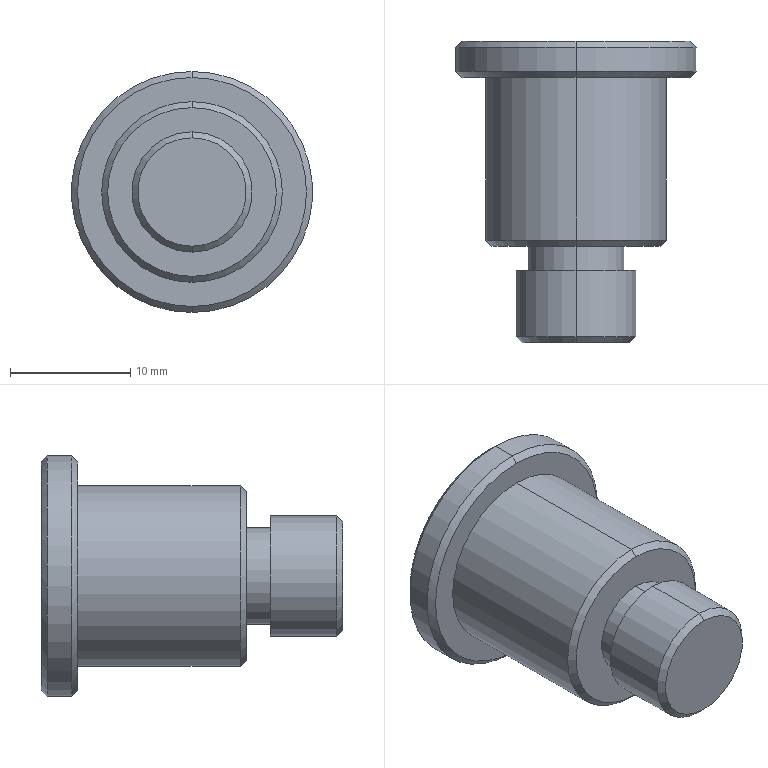Part | SolidWorks | features Chamfer 1, Revolution 1 | 1 solid | 21 faces | box 20 x 25 x 20 mm | volume 3963 mm3 | cone 8 | cylinder 8 | plane 5 | commonest cylinder face diameters 8 x2 10 x2 15 x2 20 x2
STEP:
#1=CARTESIAN_POINT('',(0.,-25.,-4.5));
#2=VERTEX_POINT('',#1);
#3=CARTESIAN_POINT('',(0.,-25.,4.5));
#4=VERTEX_POINT('',#3);
#5=CARTESIAN_POINT('',(0.,-25.,0.));
#6=DIRECTION('',(0.,-1.,0.));
#7=DIRECTION('',(0.,0.,1.));
#8=AXIS2_PLACEMENT_3D('',#5,#6,#7);
#9=CIRCLE('',#8,4.5);
#10=EDGE_CURVE('',#2,#4,#9,.T.);
#11=ORIENTED_EDGE('',*,*,#10,.F.);
#12=CARTESIAN_POINT('',(0.,-24.5,-5.));
#13=VERTEX_POINT('',#12);
#14=CARTESIAN_POINT('',(0.,-24.5,-5.));
#15=DIRECTION('',(0.,0.7071,-0.7071));
#16=VECTOR('',#15,1000.);
#17=LINE('',#14,#16);
#18=EDGE_CURVE('',#2,#13,#17,.T.);
#19=ORIENTED_EDGE('',*,*,#18,.T.);
#20=CARTESIAN_POINT('',(0.,-24.5,5.));
#21=VERTEX_POINT('',#20);
#22=CARTESIAN_POINT('',(0.,-24.5,0.));
#23=DIRECTION('',(0.,1.,0.));
#24=DIRECTION('',(0.,0.,1.));
#25=AXIS2_PLACEMENT_3D('',#22,#23,#24);
#26=CIRCLE('',#25,5.);
#27=EDGE_CURVE('',#21,#13,#26,.T.);
#28=ORIENTED_EDGE('',*,*,#27,.F.);
#29=CARTESIAN_POINT('',(0.,-24.5,5.));
#30=DIRECTION('',(0.,0.7071,0.7071));
#31=VECTOR('',#30,1000.);
#32=LINE('',#29,#31);
#33=EDGE_CURVE('',#4,#21,#32,.T.);
#34=ORIENTED_EDGE('',*,*,#33,.F.);
#35=EDGE_LOOP('',(#11,#19,#28,#34));
#36=FACE_OUTER_BOUND('',#35,.T.);
#37=CARTESIAN_POINT('',(0.,-24.5,0.));
#38=DIRECTION('',(0.,1.,0.));
#39=DIRECTION('',(0.,0.,1.));
#40=AXIS2_PLACEMENT_3D('',#37,#38,#39);
#41=CONICAL_SURFACE('',#40,5.,0.7854);
#42=ADVANCED_FACE('',(#36),#41,.T.);
#43=CARTESIAN_POINT('',(0.,-17.,-7.));
#44=VERTEX_POINT('',#43);
#45=CARTESIAN_POINT('',(0.,-17.,7.));
#46=VERTEX_POINT('',#45);
#47=CARTESIAN_POINT('',(0.,-17.,0.));
#48=DIRECTION('',(0.,-1.,0.));
#49=DIRECTION('',(0.,0.,1.));
#50=AXIS2_PLACEMENT_3D('',#47,#48,#49);
#51=CIRCLE('',#50,7.);
#52=EDGE_CURVE('',#44,#46,#51,.T.);
#53=ORIENTED_EDGE('',*,*,#52,.F.);
#54=CARTESIAN_POINT('',(0.,-16.5,-7.5));
#55=VERTEX_POINT('',#54);
#56=CARTESIAN_POINT('',(0.,-16.5,-7.5));
#57=DIRECTION('',(0.,0.7071,-0.7071));
#58=VECTOR('',#57,1000.);
#59=LINE('',#56,#58);
#60=EDGE_CURVE('',#44,#55,#59,.T.);
#61=ORIENTED_EDGE('',*,*,#60,.T.);
#62=CARTESIAN_POINT('',(0.,-16.5,7.5));
#63=VERTEX_POINT('',#62);
#64=CARTESIAN_POINT('',(0.,-16.5,0.));
#65=DIRECTION('',(0.,1.,0.));
#66=DIRECTION('',(0.,0.,1.));
#67=AXIS2_PLACEMENT_3D('',#64,#65,#66);
#68=CIRCLE('',#67,7.5);
#69=EDGE_CURVE('',#63,#55,#68,.T.);
#70=ORIENTED_EDGE('',*,*,#69,.F.);
#71=CARTESIAN_POINT('',(0.,-16.5,7.5));
#72=DIRECTION('',(0.,0.7071,0.7071));
#73=VECTOR('',#72,1000.);
#74=LINE('',#71,#73);
#75=EDGE_CURVE('',#46,#63,#74,.T.);
#76=ORIENTED_EDGE('',*,*,#75,.F.);
#77=EDGE_LOOP('',(#53,#61,#70,#76));
#78=FACE_OUTER_BOUND('',#77,.T.);
#79=CARTESIAN_POINT('',(0.,-16.5,0.));
#80=DIRECTION('',(0.,1.,0.));
#81=DIRECTION('',(0.,0.,1.));
#82=AXIS2_PLACEMENT_3D('',#79,#80,#81);
#83=CONICAL_SURFACE('',#82,7.5,0.7854);
#84=ADVANCED_FACE('',(#78),#83,.T.);
#85=CARTESIAN_POINT('',(0.,-3.,-9.5));
#86=VERTEX_POINT('',#85);
#87=CARTESIAN_POINT('',(0.,-3.,9.5));
#88=VERTEX_POINT('',#87);
#89=CARTESIAN_POINT('',(0.,-3.,0.));
#90=DIRECTION('',(0.,-1.,0.));
#91=DIRECTION('',(0.,0.,1.));
#92=AXIS2_PLACEMENT_3D('',#89,#90,#91);
#93=CIRCLE('',#92,9.5);
#94=EDGE_CURVE('',#86,#88,#93,.T.);
#95=ORIENTED_EDGE('',*,*,#94,.F.);
#96=CARTESIAN_POINT('',(0.,-2.5,-10.));
#97=VERTEX_POINT('',#96);
#98=CARTESIAN_POINT('',(0.,-2.5,-10.));
#99=DIRECTION('',(0.,0.7071,-0.7071));
#100=VECTOR('',#99,1000.);
#101=LINE('',#98,#100);
#102=EDGE_CURVE('',#86,#97,#101,.T.);
#103=ORIENTED_EDGE('',*,*,#102,.T.);
#104=CARTESIAN_POINT('',(0.,-2.5,10.));
#105=VERTEX_POINT('',#104);
#106=CARTESIAN_POINT('',(0.,-2.5,0.));
#107=DIRECTION('',(0.,1.,0.));
#108=DIRECTION('',(0.,0.,1.));
#109=AXIS2_PLACEMENT_3D('',#106,#107,#108);
#110=CIRCLE('',#109,10.);
#111=EDGE_CURVE('',#105,#97,#110,.T.);
#112=ORIENTED_EDGE('',*,*,#111,.F.);
#113=CARTESIAN_POINT('',(0.,-2.5,10.));
#114=DIRECTION('',(0.,0.7071,0.7071));
#115=VECTOR('',#114,1000.);
#116=LINE('',#113,#115);
#117=EDGE_CURVE('',#88,#105,#116,.T.);
#118=ORIENTED_EDGE('',*,*,#117,.F.);
#119=EDGE_LOOP('',(#95,#103,#112,#118));
#120=FACE_OUTER_BOUND('',#119,.T.);
#121=CARTESIAN_POINT('',(0.,-2.5,0.));
#122=DIRECTION('',(0.,1.,0.));
#123=DIRECTION('',(0.,0.,1.));
#124=AXIS2_PLACEMENT_3D('',#121,#122,#123);
#125=CONICAL_SURFACE('',#124,10.,0.7854);
#126=ADVANCED_FACE('',(#120),#125,.T.);
#127=CARTESIAN_POINT('',(0.,0.,9.5));
#128=VERTEX_POINT('',#127);
#129=CARTESIAN_POINT('',(0.,0.,-9.5));
#130=VERTEX_POINT('',#129);
#131=CARTESIAN_POINT('',(0.,0.,0.));
#132=DIRECTION('',(0.,1.,0.));
#133=DIRECTION('',(0.,0.,-1.));
#134=AXIS2_PLACEMENT_3D('',#131,#132,#133);
#135=CIRCLE('',#134,9.5);
#136=EDGE_CURVE('',#128,#130,#135,.T.);
#137=ORIENTED_EDGE('',*,*,#136,.F.);
#138=CARTESIAN_POINT('',(0.,-0.5,10.));
#139=VERTEX_POINT('',#138);
#140=CARTESIAN_POINT('',(0.,0.,9.5));
#141=DIRECTION('',(0.,-0.7071,0.7071));
#142=VECTOR('',#141,1000.);
#143=LINE('',#140,#142);
#144=EDGE_CURVE('',#128,#139,#143,.T.);
#145=ORIENTED_EDGE('',*,*,#144,.T.);
#146=CARTESIAN_POINT('',(0.,-0.5,-10.));
#147=VERTEX_POINT('',#146);
#148=CARTESIAN_POINT('',(0.,-0.5,0.));
#149=DIRECTION('',(0.,-1.,0.));
#150=DIRECTION('',(0.,0.,-1.));
#151=AXIS2_PLACEMENT_3D('',#148,#149,#150);
#152=CIRCLE('',#151,10.);
#153=EDGE_CURVE('',#147,#139,#152,.T.);
#154=ORIENTED_EDGE('',*,*,#153,.F.);
#155=CARTESIAN_POINT('',(0.,0.,-9.5));
#156=DIRECTION('',(0.,-0.7071,-0.7071));
#157=VECTOR('',#156,1000.);
#158=LINE('',#155,#157);
#159=EDGE_CURVE('',#130,#147,#158,.T.);
#160=ORIENTED_EDGE('',*,*,#159,.F.);
#161=EDGE_LOOP('',(#137,#145,#154,#160));
#162=FACE_OUTER_BOUND('',#161,.T.);
#163=CARTESIAN_POINT('',(0.,0.,0.));
#164=DIRECTION('',(0.,-1.,0.));
#165=DIRECTION('',(0.,0.,-1.));
#166=AXIS2_PLACEMENT_3D('',#163,#164,#165);
#167=CONICAL_SURFACE('',#166,9.5,0.7854);
#168=ADVANCED_FACE('',(#162),#167,.T.);
#169=ORIENTED_EDGE('',*,*,#27,.T.);
#170=CARTESIAN_POINT('',(0.,-19.,-5.));
#171=VERTEX_POINT('',#170);
#172=CARTESIAN_POINT('',(0.,0.,-5.));
#173=DIRECTION('',(0.,1.,0.));
#174=VECTOR('',#173,1000.);
#175=LINE('',#172,#174);
#176=EDGE_CURVE('',#13,#171,#175,.T.);
#177=ORIENTED_EDGE('',*,*,#176,.T.);
#178=CARTESIAN_POINT('',(0.,-19.,5.));
#179=VERTEX_POINT('',#178);
#180=CARTESIAN_POINT('',(0.,-19.,0.));
#181=DIRECTION('',(0.,1.,0.));
#182=DIRECTION('',(0.,0.,1.));
#183=AXIS2_PLACEMENT_3D('',#180,#181,#182);
#184=CIRCLE('',#183,5.);
#185=EDGE_CURVE('',#179,#171,#184,.T.);
#186=ORIENTED_EDGE('',*,*,#185,.F.);
#187=CARTESIAN_POINT('',(0.,0.,5.));
#188=DIRECTION('',(0.,1.,0.));
#189=VECTOR('',#188,1000.);
#190=LINE('',#187,#189);
#191=EDGE_CURVE('',#21,#179,#190,.T.);
#192=ORIENTED_EDGE('',*,*,#191,.F.);
#193=EDGE_LOOP('',(#169,#177,#186,#192));
#194=FACE_OUTER_BOUND('',#193,.T.);
#195=CARTESIAN_POINT('',(0.,0.,0.));
#196=DIRECTION('',(0.,1.,0.));
#197=DIRECTION('',(0.,0.,1.));
#198=AXIS2_PLACEMENT_3D('',#195,#196,#197);
#199=CYLINDRICAL_SURFACE('',#198,5.);
#200=ADVANCED_FACE('',(#194),#199,.T.);
#201=CARTESIAN_POINT('',(0.,-19.,4.));
#202=VERTEX_POINT('',#201);
#203=CARTESIAN_POINT('',(0.,-19.,-4.));
#204=VERTEX_POINT('',#203);
#205=CARTESIAN_POINT('',(0.,-19.,0.));
#206=DIRECTION('',(0.,1.,0.));
#207=DIRECTION('',(0.,0.,1.));
#208=AXIS2_PLACEMENT_3D('',#205,#206,#207);
#209=CIRCLE('',#208,4.);
#210=EDGE_CURVE('',#202,#204,#209,.T.);
#211=ORIENTED_EDGE('',*,*,#210,.T.);
#212=CARTESIAN_POINT('',(0.,-17.,-4.));
#213=VERTEX_POINT('',#212);
#214=CARTESIAN_POINT('',(0.,0.,-4.));
#215=DIRECTION('',(0.,1.,0.));
#216=VECTOR('',#215,1000.);
#217=LINE('',#214,#216);
#218=EDGE_CURVE('',#204,#213,#217,.T.);
#219=ORIENTED_EDGE('',*,*,#218,.T.);
#220=CARTESIAN_POINT('',(0.,-17.,4.));
#221=VERTEX_POINT('',#220);
#222=CARTESIAN_POINT('',(0.,-17.,0.));
#223=DIRECTION('',(0.,1.,0.));
#224=DIRECTION('',(0.,0.,1.));
#225=AXIS2_PLACEMENT_3D('',#222,#223,#224);
#226=CIRCLE('',#225,4.);
#227=EDGE_CURVE('',#221,#213,#226,.T.);
#228=ORIENTED_EDGE('',*,*,#227,.F.);
#229=CARTESIAN_POINT('',(0.,0.,4.));
#230=DIRECTION('',(0.,1.,0.));
#231=VECTOR('',#230,1000.);
#232=LINE('',#229,#231);
#233=EDGE_CURVE('',#202,#221,#232,.T.);
#234=ORIENTED_EDGE('',*,*,#233,.F.);
#235=EDGE_LOOP('',(#211,#219,#228,#234));
#236=FACE_OUTER_BOUND('',#235,.T.);
#237=CARTESIAN_POINT('',(0.,0.,0.));
#238=DIRECTION('',(0.,1.,0.));
#239=DIRECTION('',(0.,0.,1.));
#240=AXIS2_PLACEMENT_3D('',#237,#238,#239);
#241=CYLINDRICAL_SURFACE('',#240,4.);
#242=ADVANCED_FACE('',(#236),#241,.T.);
#243=ORIENTED_EDGE('',*,*,#69,.T.);
#244=CARTESIAN_POINT('',(0.,-3.,-7.5));
#245=VERTEX_POINT('',#244);
#246=CARTESIAN_POINT('',(0.,0.,-7.5));
#247=DIRECTION('',(0.,1.,0.));
#248=VECTOR('',#247,1000.);
#249=LINE('',#246,#248);
#250=EDGE_CURVE('',#55,#245,#249,.T.);
#251=ORIENTED_EDGE('',*,*,#250,.T.);
#252=CARTESIAN_POINT('',(0.,-3.,7.5));
#253=VERTEX_POINT('',#252);
#254=CARTESIAN_POINT('',(0.,-3.,0.));
#255=DIRECTION('',(0.,1.,0.));
#256=DIRECTION('',(0.,0.,1.));
#257=AXIS2_PLACEMENT_3D('',#254,#255,#256);
#258=CIRCLE('',#257,7.5);
#259=EDGE_CURVE('',#253,#245,#258,.T.);
#260=ORIENTED_EDGE('',*,*,#259,.F.);
#261=CARTESIAN_POINT('',(0.,0.,7.5));
#262=DIRECTION('',(0.,1.,0.));
#263=VECTOR('',#262,1000.);
#264=LINE('',#261,#263);
#265=EDGE_CURVE('',#63,#253,#264,.T.);
#266=ORIENTED_EDGE('',*,*,#265,.F.);
#267=EDGE_LOOP('',(#243,#251,#260,#266));
#268=FACE_OUTER_BOUND('',#267,.T.);
#269=CARTESIAN_POINT('',(0.,0.,0.));
#270=DIRECTION('',(0.,1.,0.));
#271=DIRECTION('',(0.,0.,1.));
#272=AXIS2_PLACEMENT_3D('',#269,#270,#271);
#273=CYLINDRICAL_SURFACE('',#272,7.5);
#274=ADVANCED_FACE('',(#268),#273,.T.);
#275=ORIENTED_EDGE('',*,*,#111,.T.);
#276=CARTESIAN_POINT('',(0.,0.,-10.));
#277=DIRECTION('',(0.,1.,0.));
#278=VECTOR('',#277,1000.);
#279=LINE('',#276,#278);
#280=EDGE_CURVE('',#97,#147,#279,.T.);
#281=ORIENTED_EDGE('',*,*,#280,.T.);
#282=ORIENTED_EDGE('',*,*,#153,.T.);
#283=CARTESIAN_POINT('',(0.,0.,10.));
#284=DIRECTION('',(0.,1.,0.));
#285=VECTOR('',#284,1000.);
#286=LINE('',#283,#285);
#287=EDGE_CURVE('',#105,#139,#286,.T.);
#288=ORIENTED_EDGE('',*,*,#287,.F.);
#289=EDGE_LOOP('',(#275,#281,#282,#288));
#290=FACE_OUTER_BOUND('',#289,.T.);
#291=CARTESIAN_POINT('',(0.,0.,0.));
#292=DIRECTION('',(0.,1.,0.));
#293=DIRECTION('',(0.,0.,1.));
#294=AXIS2_PLACEMENT_3D('',#291,#292,#293);
#295=CYLINDRICAL_SURFACE('',#294,10.);
#296=ADVANCED_FACE('',(#290),#295,.T.);
#297=CARTESIAN_POINT('',(0.,0.,0.));
#298=DIRECTION('',(0.,1.,0.));
#299=DIRECTION('',(0.,0.,-1.));
#300=AXIS2_PLACEMENT_3D('',#297,#298,#299);
#301=CIRCLE('',#300,9.5);
#302=EDGE_CURVE('',#130,#128,#301,.T.);
#303=ORIENTED_EDGE('',*,*,#302,.T.);
#304=ORIENTED_EDGE('',*,*,#136,.T.);
#305=EDGE_LOOP('',(#303,#304));
#306=FACE_OUTER_BOUND('',#305,.T.);
#307=CARTESIAN_POINT('',(0.,0.,0.));
#308=DIRECTION('',(0.,-1.,0.));
#309=DIRECTION('',(0.,0.,-1.));
#310=AXIS2_PLACEMENT_3D('',#307,#308,#309);
#311=PLANE('',#310);
#312=ADVANCED_FACE('',(#306),#311,.F.);
#313=ORIENTED_EDGE('',*,*,#280,.F.);
#314=CARTESIAN_POINT('',(0.,-2.5,0.));
#315=DIRECTION('',(0.,1.,0.));
#316=DIRECTION('',(0.,0.,1.));
#317=AXIS2_PLACEMENT_3D('',#314,#315,#316);
#318=CIRCLE('',#317,10.);
#319=EDGE_CURVE('',#97,#105,#318,.T.);
#320=ORIENTED_EDGE('',*,*,#319,.T.);
#321=ORIENTED_EDGE('',*,*,#287,.T.);
#322=CARTESIAN_POINT('',(0.,-0.5,0.));
#323=DIRECTION('',(0.,-1.,0.));
#324=DIRECTION('',(0.,0.,-1.));
#325=AXIS2_PLACEMENT_3D('',#322,#323,#324);
#326=CIRCLE('',#325,10.);
#327=EDGE_CURVE('',#139,#147,#326,.T.);
#328=ORIENTED_EDGE('',*,*,#327,.T.);
#329=EDGE_LOOP('',(#313,#320,#321,#328));
#330=FACE_OUTER_BOUND('',#329,.T.);
#331=CARTESIAN_POINT('',(0.,0.,0.));
#332=DIRECTION('',(0.,1.,0.));
#333=DIRECTION('',(0.,0.,1.));
#334=AXIS2_PLACEMENT_3D('',#331,#332,#333);
#335=CYLINDRICAL_SURFACE('',#334,10.);
#336=ADVANCED_FACE('',(#330),#335,.T.);
#337=CARTESIAN_POINT('',(0.,-3.,0.));
#338=DIRECTION('',(0.,-1.,0.));
#339=DIRECTION('',(0.,0.,1.));
#340=AXIS2_PLACEMENT_3D('',#337,#338,#339);
#341=CIRCLE('',#340,9.5);
#342=EDGE_CURVE('',#88,#86,#341,.T.);
#343=ORIENTED_EDGE('',*,*,#342,.T.);
#344=ORIENTED_EDGE('',*,*,#94,.T.);
#345=EDGE_LOOP('',(#343,#344));
#346=FACE_OUTER_BOUND('',#345,.T.);
#347=ORIENTED_EDGE('',*,*,#259,.T.);
#348=CARTESIAN_POINT('',(0.,-3.,0.));
#349=DIRECTION('',(0.,1.,0.));
#350=DIRECTION('',(0.,0.,1.));
#351=AXIS2_PLACEMENT_3D('',#348,#349,#350);
#352=CIRCLE('',#351,7.5);
#353=EDGE_CURVE('',#245,#253,#352,.T.);
#354=ORIENTED_EDGE('',*,*,#353,.T.);
#355=EDGE_LOOP('',(#347,#354));
#356=FACE_BOUND('',#355,.T.);
#357=CARTESIAN_POINT('',(0.,-3.,-10.));
#358=DIRECTION('',(0.,1.,0.));
#359=DIRECTION('',(0.,0.,1.));
#360=AXIS2_PLACEMENT_3D('',#357,#358,#359);
#361=PLANE('',#360);
#362=ADVANCED_FACE('',(#346,#356),#361,.F.);
#363=ORIENTED_EDGE('',*,*,#250,.F.);
#364=CARTESIAN_POINT('',(0.,-16.5,0.));
#365=DIRECTION('',(0.,1.,0.));
#366=DIRECTION('',(0.,0.,1.));
#367=AXIS2_PLACEMENT_3D('',#364,#365,#366);
#368=CIRCLE('',#367,7.5);
#369=EDGE_CURVE('',#55,#63,#368,.T.);
#370=ORIENTED_EDGE('',*,*,#369,.T.);
#371=ORIENTED_EDGE('',*,*,#265,.T.);
#372=ORIENTED_EDGE('',*,*,#353,.F.);
#373=EDGE_LOOP('',(#363,#370,#371,#372));
#374=FACE_OUTER_BOUND('',#373,.T.);
#375=CARTESIAN_POINT('',(0.,0.,0.));
#376=DIRECTION('',(0.,1.,0.));
#377=DIRECTION('',(0.,0.,1.));
#378=AXIS2_PLACEMENT_3D('',#375,#376,#377);
#379=CYLINDRICAL_SURFACE('',#378,7.5);
#380=ADVANCED_FACE('',(#374),#379,.T.);
#381=CARTESIAN_POINT('',(0.,-17.,0.));
#382=DIRECTION('',(0.,-1.,0.));
#383=DIRECTION('',(0.,0.,1.));
#384=AXIS2_PLACEMENT_3D('',#381,#382,#383);
#385=CIRCLE('',#384,7.);
#386=EDGE_CURVE('',#46,#44,#385,.T.);
#387=ORIENTED_EDGE('',*,*,#386,.T.);
#388=ORIENTED_EDGE('',*,*,#52,.T.);
#389=EDGE_LOOP('',(#387,#388));
#390=FACE_OUTER_BOUND('',#389,.T.);
#391=ORIENTED_EDGE('',*,*,#227,.T.);
#392=CARTESIAN_POINT('',(0.,-17.,0.));
#393=DIRECTION('',(0.,1.,0.));
#394=DIRECTION('',(0.,0.,1.));
#395=AXIS2_PLACEMENT_3D('',#392,#393,#394);
#396=CIRCLE('',#395,4.);
#397=EDGE_CURVE('',#213,#221,#396,.T.);
#398=ORIENTED_EDGE('',*,*,#397,.T.);
#399=EDGE_LOOP('',(#391,#398));
#400=FACE_BOUND('',#399,.T.);
#401=CARTESIAN_POINT('',(0.,-17.,-7.5));
#402=DIRECTION('',(0.,1.,0.));
#403=DIRECTION('',(0.,0.,1.));
#404=AXIS2_PLACEMENT_3D('',#401,#402,#403);
#405=PLANE('',#404);
#406=ADVANCED_FACE('',(#390,#400),#405,.F.);
#407=ORIENTED_EDGE('',*,*,#218,.F.);
#408=CARTESIAN_POINT('',(0.,-19.,0.));
#409=DIRECTION('',(0.,1.,0.));
#410=DIRECTION('',(0.,0.,1.));
#411=AXIS2_PLACEMENT_3D('',#408,#409,#410);
#412=CIRCLE('',#411,4.);
#413=EDGE_CURVE('',#204,#202,#412,.T.);
#414=ORIENTED_EDGE('',*,*,#413,.T.);
#415=ORIENTED_EDGE('',*,*,#233,.T.);
#416=ORIENTED_EDGE('',*,*,#397,.F.);
#417=EDGE_LOOP('',(#407,#414,#415,#416));
#418=FACE_OUTER_BOUND('',#417,.T.);
#419=CARTESIAN_POINT('',(0.,0.,0.));
#420=DIRECTION('',(0.,1.,0.));
#421=DIRECTION('',(0.,0.,1.));
#422=AXIS2_PLACEMENT_3D('',#419,#420,#421);
#423=CYLINDRICAL_SURFACE('',#422,4.);
#424=ADVANCED_FACE('',(#418),#423,.T.);
#425=ORIENTED_EDGE('',*,*,#210,.F.);
#426=ORIENTED_EDGE('',*,*,#413,.F.);
#427=EDGE_LOOP('',(#425,#426));
#428=FACE_BOUND('',#427,.T.);
#429=ORIENTED_EDGE('',*,*,#185,.T.);
#430=CARTESIAN_POINT('',(0.,-19.,0.));
#431=DIRECTION('',(0.,1.,0.));
#432=DIRECTION('',(0.,0.,1.));
#433=AXIS2_PLACEMENT_3D('',#430,#431,#432);
#434=CIRCLE('',#433,5.);
#435=EDGE_CURVE('',#171,#179,#434,.T.);
#436=ORIENTED_EDGE('',*,*,#435,.T.);
#437=EDGE_LOOP('',(#429,#436));
#438=FACE_OUTER_BOUND('',#437,.T.);
#439=CARTESIAN_POINT('',(0.,-19.,-4.));
#440=DIRECTION('',(0.,-1.,0.));
#441=DIRECTION('',(0.,0.,-1.));
#442=AXIS2_PLACEMENT_3D('',#439,#440,#441);
#443=PLANE('',#442);
#444=ADVANCED_FACE('',(#428,#438),#443,.F.);
#445=ORIENTED_EDGE('',*,*,#176,.F.);
#446=CARTESIAN_POINT('',(0.,-24.5,0.));
#447=DIRECTION('',(0.,1.,0.));
#448=DIRECTION('',(0.,0.,1.));
#449=AXIS2_PLACEMENT_3D('',#446,#447,#448);
#450=CIRCLE('',#449,5.);
#451=EDGE_CURVE('',#13,#21,#450,.T.);
#452=ORIENTED_EDGE('',*,*,#451,.T.);
#453=ORIENTED_EDGE('',*,*,#191,.T.);
#454=ORIENTED_EDGE('',*,*,#435,.F.);
#455=EDGE_LOOP('',(#445,#452,#453,#454));
#456=FACE_OUTER_BOUND('',#455,.T.);
#457=CARTESIAN_POINT('',(0.,0.,0.));
#458=DIRECTION('',(0.,1.,0.));
#459=DIRECTION('',(0.,0.,1.));
#460=AXIS2_PLACEMENT_3D('',#457,#458,#459);
#461=CYLINDRICAL_SURFACE('',#460,5.);
#462=ADVANCED_FACE('',(#456),#461,.T.);
#463=CARTESIAN_POINT('',(0.,-25.,0.));
#464=DIRECTION('',(0.,-1.,0.));
#465=DIRECTION('',(0.,0.,1.));
#466=AXIS2_PLACEMENT_3D('',#463,#464,#465);
#467=CIRCLE('',#466,4.5);
#468=EDGE_CURVE('',#4,#2,#467,.T.);
#469=ORIENTED_EDGE('',*,*,#468,.T.);
#470=ORIENTED_EDGE('',*,*,#10,.T.);
#471=EDGE_LOOP('',(#469,#470));
#472=FACE_OUTER_BOUND('',#471,.T.);
#473=CARTESIAN_POINT('',(0.,-25.,-5.));
#474=DIRECTION('',(0.,1.,0.));
#475=DIRECTION('',(0.,0.,1.));
#476=AXIS2_PLACEMENT_3D('',#473,#474,#475);
#477=PLANE('',#476);
#478=ADVANCED_FACE('',(#472),#477,.F.);
#479=ORIENTED_EDGE('',*,*,#144,.F.);
#480=ORIENTED_EDGE('',*,*,#302,.F.);
#481=ORIENTED_EDGE('',*,*,#159,.T.);
#482=ORIENTED_EDGE('',*,*,#327,.F.);
#483=EDGE_LOOP('',(#479,#480,#481,#482));
#484=FACE_OUTER_BOUND('',#483,.T.);
#485=CARTESIAN_POINT('',(0.,0.,0.));
#486=DIRECTION('',(0.,-1.,0.));
#487=DIRECTION('',(0.,0.,-1.));
#488=AXIS2_PLACEMENT_3D('',#485,#486,#487);
#489=CONICAL_SURFACE('',#488,9.5,0.7854);
#490=ADVANCED_FACE('',(#484),#489,.T.);
#491=ORIENTED_EDGE('',*,*,#102,.F.);
#492=ORIENTED_EDGE('',*,*,#342,.F.);
#493=ORIENTED_EDGE('',*,*,#117,.T.);
#494=ORIENTED_EDGE('',*,*,#319,.F.);
#495=EDGE_LOOP('',(#491,#492,#493,#494));
#496=FACE_OUTER_BOUND('',#495,.T.);
#497=CARTESIAN_POINT('',(0.,-2.5,0.));
#498=DIRECTION('',(0.,1.,0.));
#499=DIRECTION('',(0.,0.,1.));
#500=AXIS2_PLACEMENT_3D('',#497,#498,#499);
#501=CONICAL_SURFACE('',#500,10.,0.7854);
#502=ADVANCED_FACE('',(#496),#501,.T.);
#503=ORIENTED_EDGE('',*,*,#60,.F.);
#504=ORIENTED_EDGE('',*,*,#386,.F.);
#505=ORIENTED_EDGE('',*,*,#75,.T.);
#506=ORIENTED_EDGE('',*,*,#369,.F.);
#507=EDGE_LOOP('',(#503,#504,#505,#506));
#508=FACE_OUTER_BOUND('',#507,.T.);
#509=CARTESIAN_POINT('',(0.,-16.5,0.));
#510=DIRECTION('',(0.,1.,0.));
#511=DIRECTION('',(0.,0.,1.));
#512=AXIS2_PLACEMENT_3D('',#509,#510,#511);
#513=CONICAL_SURFACE('',#512,7.5,0.7854);
#514=ADVANCED_FACE('',(#508),#513,.T.);
#515=ORIENTED_EDGE('',*,*,#18,.F.);
#516=ORIENTED_EDGE('',*,*,#468,.F.);
#517=ORIENTED_EDGE('',*,*,#33,.T.);
#518=ORIENTED_EDGE('',*,*,#451,.F.);
#519=EDGE_LOOP('',(#515,#516,#517,#518));
#520=FACE_OUTER_BOUND('',#519,.T.);
#521=CARTESIAN_POINT('',(0.,-24.5,0.));
#522=DIRECTION('',(0.,1.,0.));
#523=DIRECTION('',(0.,0.,1.));
#524=AXIS2_PLACEMENT_3D('',#521,#522,#523);
#525=CONICAL_SURFACE('',#524,5.,0.7854);
#526=ADVANCED_FACE('',(#520),#525,.T.);
#527=CLOSED_SHELL('',(#42,#84,#126,#168,#200,#242,#274,#296,#312,#336,#362,#380,#406,#424,#444,#462,#478,#490,#502,#514,#526));
#528=MANIFOLD_SOLID_BREP('',#527);
#529=CARTESIAN_POINT('',(0.,0.,0.));
#530=DIRECTION('',(0.,0.,1.));
#531=DIRECTION('',(1.,0.,0.));
#532=AXIS2_PLACEMENT_3D('',#529,#530,#531);
#533=(LENGTH_UNIT()NAMED_UNIT(*)SI_UNIT(.MILLI.,.METRE.));
#534=UNCERTAINTY_MEASURE_WITH_UNIT(LENGTH_MEASURE(0.00001),#533,'','');
#535=(NAMED_UNIT(*)PLANE_ANGLE_UNIT()SI_UNIT($,.RADIAN.));
#536=(NAMED_UNIT(*)SI_UNIT($,.STERADIAN.)SOLID_ANGLE_UNIT());
#537=(GEOMETRIC_REPRESENTATION_CONTEXT(3)GLOBAL_UNCERTAINTY_ASSIGNED_CONTEXT((#534))GLOBAL_UNIT_ASSIGNED_CONTEXT((#533,#535,#536))REPRESENTATION_CONTEXT('',''));
#538=ADVANCED_BREP_SHAPE_REPRESENTATION('',(#528,#532),#537);